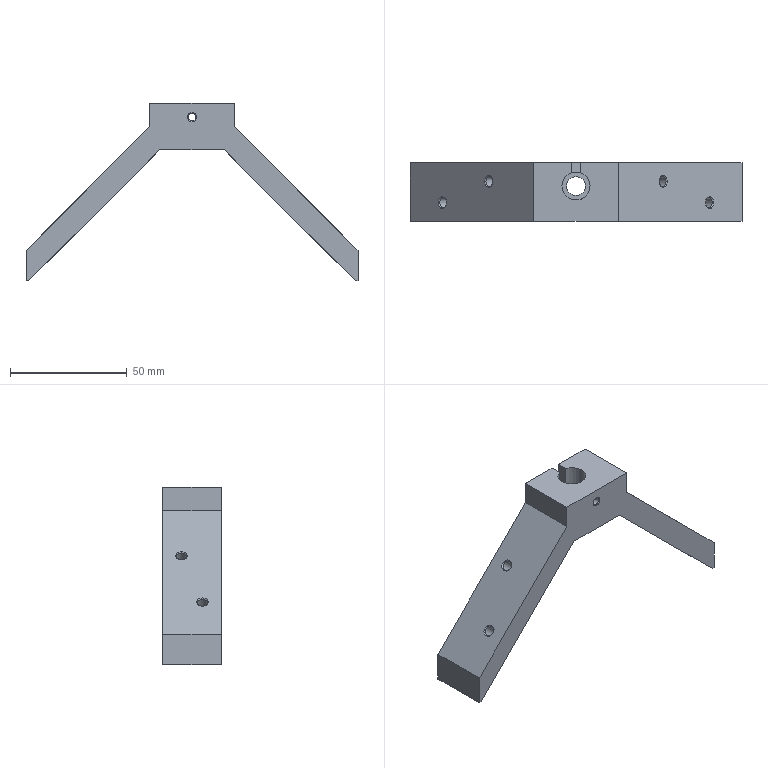Part | NX | features DATUM_CSYS 8, SKETCH 7, SIMPLE HOLE 5, SYMBOLIC_THREAD 5, HOLE PACKAGE 4, EXTRUDE 3, EXTRACT_FACE 2, CBORE_HOLE 1, Instance Feature 1, Mirror Feature 1 | 1 solid | 35 faces | box 142 x 25 x 76 mm | volume 53307 mm3 | plane 18 | cone 9 | cylinder 7 | spline 1 | commonest cylinder face diameters 4.2 x4 3.3 x1 8 x1 12 x1
STEP:
#1=CARTESIAN_POINT('',(2.,12.5,20.));
#2=VERTEX_POINT('',#1);
#3=CARTESIAN_POINT('',(2.,12.5,10.));
#4=VERTEX_POINT('',#3);
#5=CARTESIAN_POINT('',(2.,12.5,20.));
#6=DIRECTION('',(0.,0.,-1.));
#7=VECTOR('',#6,1000.);
#8=LINE('',#5,#7);
#9=EDGE_CURVE('',#2,#4,#8,.T.);
#10=ORIENTED_EDGE('',*,*,#9,.F.);
#11=CARTESIAN_POINT('',(18.,12.5,20.));
#12=VERTEX_POINT('',#11);
#13=CARTESIAN_POINT('',(18.,12.5,20.));
#14=DIRECTION('',(-1.,0.,0.));
#15=VECTOR('',#14,1000.);
#16=LINE('',#13,#15);
#17=EDGE_CURVE('',#12,#2,#16,.T.);
#18=ORIENTED_EDGE('',*,*,#17,.F.);
#19=CARTESIAN_POINT('',(18.,12.5,10.));
#20=VERTEX_POINT('',#19);
#21=CARTESIAN_POINT('',(18.,12.5,20.));
#22=DIRECTION('',(0.,0.,-1.));
#23=VECTOR('',#22,1000.);
#24=LINE('',#21,#23);
#25=EDGE_CURVE('',#12,#20,#24,.T.);
#26=ORIENTED_EDGE('',*,*,#25,.T.);
#27=CARTESIAN_POINT('',(71.,12.5,-43.));
#28=VERTEX_POINT('',#27);
#29=CARTESIAN_POINT('',(71.,12.5,-43.));
#30=DIRECTION('',(-0.7071,0.,0.7071));
#31=VECTOR('',#30,1000.);
#32=LINE('',#29,#31);
#33=EDGE_CURVE('',#28,#20,#32,.T.);
#34=ORIENTED_EDGE('',*,*,#33,.F.);
#35=CARTESIAN_POINT('',(71.,12.5,-56.));
#36=VERTEX_POINT('',#35);
#37=CARTESIAN_POINT('',(71.,12.5,-56.));
#38=DIRECTION('',(0.,0.,1.));
#39=VECTOR('',#38,1000.);
#40=LINE('',#37,#39);
#41=EDGE_CURVE('',#36,#28,#40,.T.);
#42=ORIENTED_EDGE('',*,*,#41,.F.);
#43=CARTESIAN_POINT('',(69.858,12.5,-56.));
#44=VERTEX_POINT('',#43);
#45=CARTESIAN_POINT('',(69.858,12.5,-56.));
#46=DIRECTION('',(1.,0.,0.));
#47=VECTOR('',#46,1000.);
#48=LINE('',#45,#47);
#49=EDGE_CURVE('',#44,#36,#48,.T.);
#50=ORIENTED_EDGE('',*,*,#49,.F.);
#51=CARTESIAN_POINT('',(13.858,12.5,0.));
#52=VERTEX_POINT('',#51);
#53=CARTESIAN_POINT('',(13.858,12.5,0.));
#54=DIRECTION('',(0.7071,0.,-0.7071));
#55=VECTOR('',#54,1000.);
#56=LINE('',#53,#55);
#57=EDGE_CURVE('',#52,#44,#56,.T.);
#58=ORIENTED_EDGE('',*,*,#57,.F.);
#59=CARTESIAN_POINT('',(-13.858,12.5,0.));
#60=VERTEX_POINT('',#59);
#61=CARTESIAN_POINT('',(18.,12.5,0.));
#62=DIRECTION('',(-1.,0.,0.));
#63=VECTOR('',#62,1000.);
#64=LINE('',#61,#63);
#65=EDGE_CURVE('',#52,#60,#64,.T.);
#66=ORIENTED_EDGE('',*,*,#65,.T.);
#67=CARTESIAN_POINT('',(-69.858,12.5,-56.));
#68=VERTEX_POINT('',#67);
#69=CARTESIAN_POINT('',(-69.858,12.5,-56.));
#70=DIRECTION('',(0.7071,0.,0.7071));
#71=VECTOR('',#70,1000.);
#72=LINE('',#69,#71);
#73=EDGE_CURVE('',#68,#60,#72,.T.);
#74=ORIENTED_EDGE('',*,*,#73,.F.);
#75=CARTESIAN_POINT('',(-71.,12.5,-56.));
#76=VERTEX_POINT('',#75);
#77=CARTESIAN_POINT('',(-71.,12.5,-56.));
#78=DIRECTION('',(1.,0.,0.));
#79=VECTOR('',#78,1000.);
#80=LINE('',#77,#79);
#81=EDGE_CURVE('',#76,#68,#80,.T.);
#82=ORIENTED_EDGE('',*,*,#81,.F.);
#83=CARTESIAN_POINT('',(-71.,12.5,-43.));
#84=VERTEX_POINT('',#83);
#85=CARTESIAN_POINT('',(-71.,12.5,-43.));
#86=DIRECTION('',(0.,0.,-1.));
#87=VECTOR('',#86,1000.);
#88=LINE('',#85,#87);
#89=EDGE_CURVE('',#84,#76,#88,.T.);
#90=ORIENTED_EDGE('',*,*,#89,.F.);
#91=CARTESIAN_POINT('',(-18.,12.5,10.));
#92=VERTEX_POINT('',#91);
#93=CARTESIAN_POINT('',(-18.,12.5,10.));
#94=DIRECTION('',(-0.7071,0.,-0.7071));
#95=VECTOR('',#94,1000.);
#96=LINE('',#93,#95);
#97=EDGE_CURVE('',#92,#84,#96,.T.);
#98=ORIENTED_EDGE('',*,*,#97,.F.);
#99=CARTESIAN_POINT('',(-18.,12.5,20.));
#100=VERTEX_POINT('',#99);
#101=CARTESIAN_POINT('',(-18.,12.5,20.));
#102=DIRECTION('',(0.,0.,-1.));
#103=VECTOR('',#102,1000.);
#104=LINE('',#101,#103);
#105=EDGE_CURVE('',#100,#92,#104,.T.);
#106=ORIENTED_EDGE('',*,*,#105,.F.);
#107=CARTESIAN_POINT('',(-2.,12.5,20.));
#108=VERTEX_POINT('',#107);
#109=CARTESIAN_POINT('',(18.,12.5,20.));
#110=DIRECTION('',(-1.,0.,0.));
#111=VECTOR('',#110,1000.);
#112=LINE('',#109,#111);
#113=EDGE_CURVE('',#108,#100,#112,.T.);
#114=ORIENTED_EDGE('',*,*,#113,.F.);
#115=CARTESIAN_POINT('',(-2.,12.5,10.));
#116=VERTEX_POINT('',#115);
#117=CARTESIAN_POINT('',(-2.,12.5,20.));
#118=DIRECTION('',(0.,0.,1.));
#119=VECTOR('',#118,1000.);
#120=LINE('',#117,#119);
#121=EDGE_CURVE('',#116,#108,#120,.T.);
#122=ORIENTED_EDGE('',*,*,#121,.F.);
#123=CARTESIAN_POINT('',(18.,12.5,10.));
#124=DIRECTION('',(1.,0.,0.));
#125=VECTOR('',#124,1000.);
#126=LINE('',#123,#125);
#127=EDGE_CURVE('',#116,#4,#126,.T.);
#128=ORIENTED_EDGE('',*,*,#127,.T.);
#129=EDGE_LOOP('',(#10,#18,#26,#34,#42,#50,#58,#66,#74,#82,#90,#98,#106,#114,#122,#128));
#130=FACE_BOUND('',#129,.T.);
#131=CARTESIAN_POINT('',(18.,12.5,20.));
#132=DIRECTION('',(0.,-1.,0.));
#133=DIRECTION('',(0.,0.,-1.));
#134=AXIS2_PLACEMENT_3D('',#131,#132,#133);
#135=PLANE('',#134);
#136=ADVANCED_FACE('',(#130),#135,.F.);
#137=CARTESIAN_POINT('',(2.,8.157,20.));
#138=VERTEX_POINT('',#137);
#139=CARTESIAN_POINT('',(-2.,8.157,20.));
#140=VERTEX_POINT('',#139);
#141=CARTESIAN_POINT('',(0.,2.5,20.));
#142=DIRECTION('',(0.,0.,-1.));
#143=DIRECTION('',(-1.,0.,0.));
#144=AXIS2_PLACEMENT_3D('',#141,#142,#143);
#145=CIRCLE('',#144,6.);
#146=EDGE_CURVE('',#138,#140,#145,.T.);
#147=ORIENTED_EDGE('',*,*,#146,.T.);
#148=CARTESIAN_POINT('',(-2.,5.4,20.));
#149=DIRECTION('',(0.,1.,0.));
#150=VECTOR('',#149,1000.);
#151=LINE('',#148,#150);
#152=EDGE_CURVE('',#140,#108,#151,.T.);
#153=ORIENTED_EDGE('',*,*,#152,.T.);
#154=ORIENTED_EDGE('',*,*,#113,.T.);
#155=CARTESIAN_POINT('',(-18.,-12.5,20.));
#156=VERTEX_POINT('',#155);
#157=CARTESIAN_POINT('',(-18.,12.5,20.));
#158=DIRECTION('',(0.,-1.,0.));
#159=VECTOR('',#158,1000.);
#160=LINE('',#157,#159);
#161=EDGE_CURVE('',#100,#156,#160,.T.);
#162=ORIENTED_EDGE('',*,*,#161,.T.);
#163=CARTESIAN_POINT('',(18.,-12.5,20.));
#164=VERTEX_POINT('',#163);
#165=CARTESIAN_POINT('',(-18.,-12.5,20.));
#166=DIRECTION('',(1.,0.,0.));
#167=VECTOR('',#166,1000.);
#168=LINE('',#165,#167);
#169=EDGE_CURVE('',#156,#164,#168,.T.);
#170=ORIENTED_EDGE('',*,*,#169,.T.);
#171=CARTESIAN_POINT('',(18.,-12.5,20.));
#172=DIRECTION('',(0.,1.,0.));
#173=VECTOR('',#172,1000.);
#174=LINE('',#171,#173);
#175=EDGE_CURVE('',#164,#12,#174,.T.);
#176=ORIENTED_EDGE('',*,*,#175,.T.);
#177=ORIENTED_EDGE('',*,*,#17,.T.);
#178=CARTESIAN_POINT('',(2.,14.3,20.));
#179=DIRECTION('',(0.,-1.,0.));
#180=VECTOR('',#179,1000.);
#181=LINE('',#178,#180);
#182=EDGE_CURVE('',#2,#138,#181,.T.);
#183=ORIENTED_EDGE('',*,*,#182,.T.);
#184=EDGE_LOOP('',(#147,#153,#154,#162,#170,#176,#177,#183));
#185=FACE_BOUND('',#184,.T.);
#186=CARTESIAN_POINT('',(0.,0.,20.));
#187=DIRECTION('',(0.,0.,1.));
#188=DIRECTION('',(1.,0.,0.));
#189=AXIS2_PLACEMENT_3D('',#186,#187,#188);
#190=PLANE('',#189);
#191=ADVANCED_FACE('',(#185),#190,.T.);
#192=CARTESIAN_POINT('',(-6.,2.5,8.));
#193=VERTEX_POINT('',#192);
#194=CARTESIAN_POINT('',(0.,2.5,8.));
#195=DIRECTION('',(0.,0.,-1.));
#196=DIRECTION('',(-1.,0.,0.));
#197=AXIS2_PLACEMENT_3D('',#194,#195,#196);
#198=CIRCLE('',#197,6.);
#199=EDGE_CURVE('',#193,#193,#198,.F.);
#200=ORIENTED_EDGE('',*,*,#199,.F.);
#201=EDGE_LOOP('',(#200));
#202=FACE_BOUND('',#201,.T.);
#203=CARTESIAN_POINT('',(0.,-3.5,16.061));
#204=VERTEX_POINT('',#203);
#205=CARTESIAN_POINT('',(1.275,-3.383,15.709));
#206=CARTESIAN_POINT('',(0.03766,-3.572,16.278));
#207=CARTESIAN_POINT('',(-1.209,-3.398,15.751));
#208=CARTESIAN_POINT('',(-1.79,-3.229,14.866));
#209=CARTESIAN_POINT('',(-1.965,-3.169,14.045));
#210=CARTESIAN_POINT('',(-1.824,-3.218,13.231));
#211=CARTESIAN_POINT('',(-1.288,-3.378,12.314));
#212=CARTESIAN_POINT('',(-0.07795,-3.571,11.724));
#213=CARTESIAN_POINT('',(1.193,-3.403,12.223));
#214=CARTESIAN_POINT('',(1.789,-3.229,13.134));
#215=CARTESIAN_POINT('',(1.965,-3.169,13.957));
#216=CARTESIAN_POINT('',(1.824,-3.218,14.771));
#217=CARTESIAN_POINT('',(1.275,-3.383,15.709));
#218=CARTESIAN_POINT('',(0.03766,-3.572,16.278));
#219=CARTESIAN_POINT('',(-1.209,-3.398,15.751));
#220=B_SPLINE_CURVE_WITH_KNOTS('',3,(#205,#206,#207,#208,#209,#210,#211,#212,#213,#214,#215,#216,#217,#218,#219),.UNSPECIFIED.,.T.,.F.,(1,1,1,1,1,1,1,1,1,1,1,1,1,1,1,1,1,1,1),(-0.2533,-0.1908,-0.1283,0.,0.1187,0.1841,0.2467,0.3092,0.3717,0.4936,0.6184,0.684,0.7467,0.8092,0.8717,1.,1.119,1.184,1.247),.UNSPECIFIED.);
#221=EDGE_CURVE('',#204,#204,#220,.T.);
#222=ORIENTED_EDGE('',*,*,#221,.T.);
#223=EDGE_LOOP('',(#222));
#224=FACE_BOUND('',#223,.T.);
#225=CARTESIAN_POINT('',(2.,8.157,10.));
#226=VERTEX_POINT('',#225);
#227=CARTESIAN_POINT('',(2.,8.157,20.));
#228=DIRECTION('',(0.,0.,-1.));
#229=VECTOR('',#228,1000.);
#230=LINE('',#227,#229);
#231=EDGE_CURVE('',#226,#138,#230,.F.);
#232=ORIENTED_EDGE('',*,*,#231,.F.);
#233=CARTESIAN_POINT('',(-2.,8.157,10.));
#234=VERTEX_POINT('',#233);
#235=CARTESIAN_POINT('',(0.,2.5,10.));
#236=DIRECTION('',(0.,0.,-1.));
#237=DIRECTION('',(-1.,0.,0.));
#238=AXIS2_PLACEMENT_3D('',#235,#236,#237);
#239=CIRCLE('',#238,6.);
#240=EDGE_CURVE('',#226,#234,#239,.F.);
#241=ORIENTED_EDGE('',*,*,#240,.T.);
#242=CARTESIAN_POINT('',(-2.,8.157,20.));
#243=DIRECTION('',(0.,0.,-1.));
#244=VECTOR('',#243,1000.);
#245=LINE('',#242,#244);
#246=EDGE_CURVE('',#140,#234,#245,.T.);
#247=ORIENTED_EDGE('',*,*,#246,.F.);
#248=ORIENTED_EDGE('',*,*,#146,.F.);
#249=EDGE_LOOP('',(#232,#241,#247,#248));
#250=FACE_BOUND('',#249,.T.);
#251=CARTESIAN_POINT('',(0.,2.5,20.));
#252=DIRECTION('',(0.,0.,-1.));
#253=DIRECTION('',(-1.,0.,0.));
#254=AXIS2_PLACEMENT_3D('',#251,#252,#253);
#255=CYLINDRICAL_SURFACE('',#254,6.);
#256=ADVANCED_FACE('',(#202,#224,#250),#255,.F.);
#257=CARTESIAN_POINT('',(4.,2.5,0.));
#258=VERTEX_POINT('',#257);
#259=CARTESIAN_POINT('',(0.,2.5,0.));
#260=DIRECTION('',(0.,0.,1.));
#261=DIRECTION('',(1.,0.,0.));
#262=AXIS2_PLACEMENT_3D('',#259,#260,#261);
#263=CIRCLE('',#262,4.);
#264=EDGE_CURVE('',#258,#258,#263,.T.);
#265=ORIENTED_EDGE('',*,*,#264,.T.);
#266=EDGE_LOOP('',(#265));
#267=FACE_BOUND('',#266,.T.);
#268=CARTESIAN_POINT('',(13.858,-12.5,0.));
#269=VERTEX_POINT('',#268);
#270=CARTESIAN_POINT('',(13.858,-12.5,0.));
#271=DIRECTION('',(0.,1.,0.));
#272=VECTOR('',#271,1000.);
#273=LINE('',#270,#272);
#274=EDGE_CURVE('',#269,#52,#273,.T.);
#275=ORIENTED_EDGE('',*,*,#274,.F.);
#276=CARTESIAN_POINT('',(-13.858,-12.5,0.));
#277=VERTEX_POINT('',#276);
#278=CARTESIAN_POINT('',(-18.,-12.5,0.));
#279=DIRECTION('',(1.,0.,0.));
#280=VECTOR('',#279,1000.);
#281=LINE('',#278,#280);
#282=EDGE_CURVE('',#277,#269,#281,.T.);
#283=ORIENTED_EDGE('',*,*,#282,.F.);
#284=CARTESIAN_POINT('',(-13.858,-12.5,0.));
#285=DIRECTION('',(0.,1.,0.));
#286=VECTOR('',#285,1000.);
#287=LINE('',#284,#286);
#288=EDGE_CURVE('',#277,#60,#287,.T.);
#289=ORIENTED_EDGE('',*,*,#288,.T.);
#290=ORIENTED_EDGE('',*,*,#65,.F.);
#291=EDGE_LOOP('',(#275,#283,#289,#290));
#292=FACE_BOUND('',#291,.T.);
#293=CARTESIAN_POINT('',(0.,0.,0.));
#294=DIRECTION('',(0.,0.,1.));
#295=DIRECTION('',(1.,0.,0.));
#296=AXIS2_PLACEMENT_3D('',#293,#294,#295);
#297=PLANE('',#296);
#298=ADVANCED_FACE('',(#267,#292),#297,.F.);
#299=CARTESIAN_POINT('',(18.,-12.5,10.));
#300=VERTEX_POINT('',#299);
#301=CARTESIAN_POINT('',(18.,-12.5,10.));
#302=DIRECTION('',(0.,1.,0.));
#303=VECTOR('',#302,1000.);
#304=LINE('',#301,#303);
#305=EDGE_CURVE('',#300,#20,#304,.T.);
#306=ORIENTED_EDGE('',*,*,#305,.T.);
#307=ORIENTED_EDGE('',*,*,#25,.F.);
#308=ORIENTED_EDGE('',*,*,#175,.F.);
#309=CARTESIAN_POINT('',(18.,-12.5,20.));
#310=DIRECTION('',(0.,0.,-1.));
#311=VECTOR('',#310,1000.);
#312=LINE('',#309,#311);
#313=EDGE_CURVE('',#164,#300,#312,.T.);
#314=ORIENTED_EDGE('',*,*,#313,.T.);
#315=EDGE_LOOP('',(#306,#307,#308,#314));
#316=FACE_BOUND('',#315,.T.);
#317=CARTESIAN_POINT('',(18.,-12.5,20.));
#318=DIRECTION('',(-1.,0.,0.));
#319=DIRECTION('',(0.,0.,1.));
#320=AXIS2_PLACEMENT_3D('',#317,#318,#319);
#321=PLANE('',#320);
#322=ADVANCED_FACE('',(#316),#321,.F.);
#323=CARTESIAN_POINT('',(-18.,-12.5,10.));
#324=VERTEX_POINT('',#323);
#325=CARTESIAN_POINT('',(-18.,-12.5,10.));
#326=DIRECTION('',(0.,1.,0.));
#327=VECTOR('',#326,1000.);
#328=LINE('',#325,#327);
#329=EDGE_CURVE('',#324,#92,#328,.T.);
#330=ORIENTED_EDGE('',*,*,#329,.F.);
#331=CARTESIAN_POINT('',(-18.,-12.5,20.));
#332=DIRECTION('',(0.,0.,-1.));
#333=VECTOR('',#332,1000.);
#334=LINE('',#331,#333);
#335=EDGE_CURVE('',#156,#324,#334,.T.);
#336=ORIENTED_EDGE('',*,*,#335,.F.);
#337=ORIENTED_EDGE('',*,*,#161,.F.);
#338=ORIENTED_EDGE('',*,*,#105,.T.);
#339=EDGE_LOOP('',(#330,#336,#337,#338));
#340=FACE_BOUND('',#339,.T.);
#341=CARTESIAN_POINT('',(-18.,12.5,20.));
#342=DIRECTION('',(1.,0.,0.));
#343=DIRECTION('',(0.,0.,-1.));
#344=AXIS2_PLACEMENT_3D('',#341,#342,#343);
#345=PLANE('',#344);
#346=ADVANCED_FACE('',(#340),#345,.F.);
#347=CARTESIAN_POINT('',(0.,-12.5,16.));
#348=VERTEX_POINT('',#347);
#349=CARTESIAN_POINT('',(0.,-12.5,14.));
#350=DIRECTION('',(0.,1.,0.));
#351=DIRECTION('',(0.,0.,1.));
#352=AXIS2_PLACEMENT_3D('',#349,#350,#351);
#353=CIRCLE('',#352,2.);
#354=EDGE_CURVE('',#348,#348,#353,.T.);
#355=ORIENTED_EDGE('',*,*,#354,.T.);
#356=EDGE_LOOP('',(#355));
#357=FACE_BOUND('',#356,.T.);
#358=ORIENTED_EDGE('',*,*,#282,.T.);
#359=CARTESIAN_POINT('',(69.858,-12.5,-56.));
#360=VERTEX_POINT('',#359);
#361=CARTESIAN_POINT('',(13.858,-12.5,0.));
#362=DIRECTION('',(0.7071,0.,-0.7071));
#363=VECTOR('',#362,1000.);
#364=LINE('',#361,#363);
#365=EDGE_CURVE('',#269,#360,#364,.T.);
#366=ORIENTED_EDGE('',*,*,#365,.T.);
#367=CARTESIAN_POINT('',(71.,-12.5,-56.));
#368=VERTEX_POINT('',#367);
#369=CARTESIAN_POINT('',(69.858,-12.5,-56.));
#370=DIRECTION('',(1.,0.,0.));
#371=VECTOR('',#370,1000.);
#372=LINE('',#369,#371);
#373=EDGE_CURVE('',#360,#368,#372,.T.);
#374=ORIENTED_EDGE('',*,*,#373,.T.);
#375=CARTESIAN_POINT('',(71.,-12.5,-43.));
#376=VERTEX_POINT('',#375);
#377=CARTESIAN_POINT('',(71.,-12.5,-56.));
#378=DIRECTION('',(0.,0.,1.));
#379=VECTOR('',#378,1000.);
#380=LINE('',#377,#379);
#381=EDGE_CURVE('',#368,#376,#380,.T.);
#382=ORIENTED_EDGE('',*,*,#381,.T.);
#383=CARTESIAN_POINT('',(71.,-12.5,-43.));
#384=DIRECTION('',(-0.7071,0.,0.7071));
#385=VECTOR('',#384,1000.);
#386=LINE('',#383,#385);
#387=EDGE_CURVE('',#376,#300,#386,.T.);
#388=ORIENTED_EDGE('',*,*,#387,.T.);
#389=ORIENTED_EDGE('',*,*,#313,.F.);
#390=ORIENTED_EDGE('',*,*,#169,.F.);
#391=ORIENTED_EDGE('',*,*,#335,.T.);
#392=CARTESIAN_POINT('',(-71.,-12.5,-43.));
#393=VERTEX_POINT('',#392);
#394=CARTESIAN_POINT('',(-18.,-12.5,10.));
#395=DIRECTION('',(-0.7071,0.,-0.7071));
#396=VECTOR('',#395,1000.);
#397=LINE('',#394,#396);
#398=EDGE_CURVE('',#324,#393,#397,.T.);
#399=ORIENTED_EDGE('',*,*,#398,.T.);
#400=CARTESIAN_POINT('',(-71.,-12.5,-56.));
#401=VERTEX_POINT('',#400);
#402=CARTESIAN_POINT('',(-71.,-12.5,-43.));
#403=DIRECTION('',(0.,0.,-1.));
#404=VECTOR('',#403,1000.);
#405=LINE('',#402,#404);
#406=EDGE_CURVE('',#393,#401,#405,.T.);
#407=ORIENTED_EDGE('',*,*,#406,.T.);
#408=CARTESIAN_POINT('',(-69.858,-12.5,-56.));
#409=VERTEX_POINT('',#408);
#410=CARTESIAN_POINT('',(-71.,-12.5,-56.));
#411=DIRECTION('',(1.,0.,0.));
#412=VECTOR('',#411,1000.);
#413=LINE('',#410,#412);
#414=EDGE_CURVE('',#401,#409,#413,.T.);
#415=ORIENTED_EDGE('',*,*,#414,.T.);
#416=CARTESIAN_POINT('',(-69.858,-12.5,-56.));
#417=DIRECTION('',(0.7071,0.,0.7071));
#418=VECTOR('',#417,1000.);
#419=LINE('',#416,#418);
#420=EDGE_CURVE('',#409,#277,#419,.T.);
#421=ORIENTED_EDGE('',*,*,#420,.T.);
#422=EDGE_LOOP('',(#358,#366,#374,#382,#388,#389,#390,#391,#399,#407,#415,#421));
#423=FACE_BOUND('',#422,.T.);
#424=CARTESIAN_POINT('',(-18.,-12.5,20.));
#425=DIRECTION('',(0.,1.,0.));
#426=DIRECTION('',(0.,0.,1.));
#427=AXIS2_PLACEMENT_3D('',#424,#425,#426);
#428=PLANE('',#427);
#429=ADVANCED_FACE('',(#357,#423),#428,.F.);
#430=ORIENTED_EDGE('',*,*,#89,.T.);
#431=CARTESIAN_POINT('',(-71.,-12.5,-56.));
#432=DIRECTION('',(0.,1.,0.));
#433=VECTOR('',#432,1000.);
#434=LINE('',#431,#433);
#435=EDGE_CURVE('',#401,#76,#434,.T.);
#436=ORIENTED_EDGE('',*,*,#435,.F.);
#437=ORIENTED_EDGE('',*,*,#406,.F.);
#438=CARTESIAN_POINT('',(-71.,-12.5,-43.));
#439=DIRECTION('',(0.,1.,0.));
#440=VECTOR('',#439,1000.);
#441=LINE('',#438,#440);
#442=EDGE_CURVE('',#393,#84,#441,.T.);
#443=ORIENTED_EDGE('',*,*,#442,.T.);
#444=EDGE_LOOP('',(#430,#436,#437,#443));
#445=FACE_BOUND('',#444,.T.);
#446=CARTESIAN_POINT('',(-71.,-12.5,-43.));
#447=DIRECTION('',(1.,0.,0.));
#448=DIRECTION('',(0.,0.,-1.));
#449=AXIS2_PLACEMENT_3D('',#446,#447,#448);
#450=PLANE('',#449);
#451=ADVANCED_FACE('',(#445),#450,.F.);
#452=ORIENTED_EDGE('',*,*,#81,.T.);
#453=CARTESIAN_POINT('',(-69.858,-12.5,-56.));
#454=DIRECTION('',(0.,1.,0.));
#455=VECTOR('',#454,1000.);
#456=LINE('',#453,#455);
#457=EDGE_CURVE('',#409,#68,#456,.T.);
#458=ORIENTED_EDGE('',*,*,#457,.F.);
#459=ORIENTED_EDGE('',*,*,#414,.F.);
#460=ORIENTED_EDGE('',*,*,#435,.T.);
#461=EDGE_LOOP('',(#452,#458,#459,#460));
#462=FACE_BOUND('',#461,.T.);
#463=CARTESIAN_POINT('',(-71.,-12.5,-56.));
#464=DIRECTION('',(0.,0.,1.));
#465=DIRECTION('',(1.,0.,0.));
#466=AXIS2_PLACEMENT_3D('',#463,#464,#465);
#467=PLANE('',#466);
#468=ADVANCED_FACE('',(#462),#467,.F.);
#469=CARTESIAN_POINT('',(-48.291,-4.5,-34.433));
#470=VERTEX_POINT('',#469);
#471=CARTESIAN_POINT('',(-50.059,-4.5,-36.201));
#472=DIRECTION('',(-0.7071,0.,0.7071));
#473=DIRECTION('',(0.7071,0.,0.7071));
#474=AXIS2_PLACEMENT_3D('',#471,#472,#473);
#475=CIRCLE('',#474,2.5);
#476=EDGE_CURVE('',#470,#470,#475,.T.);
#477=ORIENTED_EDGE('',*,*,#476,.T.);
#478=EDGE_LOOP('',(#477));
#479=FACE_BOUND('',#478,.T.);
#480=CARTESIAN_POINT('',(-28.492,4.5,-14.634));
#481=VERTEX_POINT('',#480);
#482=CARTESIAN_POINT('',(-30.26,4.5,-16.402));
#483=DIRECTION('',(-0.7071,0.,0.7071));
#484=DIRECTION('',(0.7071,0.,0.7071));
#485=AXIS2_PLACEMENT_3D('',#482,#483,#484);
#486=CIRCLE('',#485,2.5);
#487=EDGE_CURVE('',#481,#481,#486,.T.);
#488=ORIENTED_EDGE('',*,*,#487,.T.);
#489=EDGE_LOOP('',(#488));
#490=FACE_BOUND('',#489,.T.);
#491=ORIENTED_EDGE('',*,*,#73,.T.);
#492=ORIENTED_EDGE('',*,*,#288,.F.);
#493=ORIENTED_EDGE('',*,*,#420,.F.);
#494=ORIENTED_EDGE('',*,*,#457,.T.);
#495=EDGE_LOOP('',(#491,#492,#493,#494));
#496=FACE_BOUND('',#495,.T.);
#497=CARTESIAN_POINT('',(-69.858,-12.5,-56.));
#498=DIRECTION('',(-0.7071,0.,0.7071));
#499=DIRECTION('',(0.7071,0.,0.7071));
#500=AXIS2_PLACEMENT_3D('',#497,#498,#499);
#501=PLANE('',#500);
#502=ADVANCED_FACE('',(#479,#490,#496),#501,.F.);
#503=CARTESIAN_POINT('',(-58.898,-4.5,-30.898));
#504=VERTEX_POINT('',#503);
#505=CARTESIAN_POINT('',(-57.13,-4.5,-29.13));
#506=DIRECTION('',(0.7071,0.,-0.7071));
#507=DIRECTION('',(-0.7071,0.,-0.7071));
#508=AXIS2_PLACEMENT_3D('',#505,#506,#507);
#509=CIRCLE('',#508,2.5);
#510=EDGE_CURVE('',#504,#504,#509,.T.);
#511=ORIENTED_EDGE('',*,*,#510,.T.);
#512=EDGE_LOOP('',(#511));
#513=FACE_BOUND('',#512,.T.);
#514=CARTESIAN_POINT('',(-39.099,4.5,-11.099));
#515=VERTEX_POINT('',#514);
#516=CARTESIAN_POINT('',(-37.331,4.5,-9.331));
#517=DIRECTION('',(0.7071,0.,-0.7071));
#518=DIRECTION('',(-0.7071,0.,-0.7071));
#519=AXIS2_PLACEMENT_3D('',#516,#517,#518);
#520=CIRCLE('',#519,2.5);
#521=EDGE_CURVE('',#515,#515,#520,.T.);
#522=ORIENTED_EDGE('',*,*,#521,.T.);
#523=EDGE_LOOP('',(#522));
#524=FACE_BOUND('',#523,.T.);
#525=ORIENTED_EDGE('',*,*,#97,.T.);
#526=ORIENTED_EDGE('',*,*,#442,.F.);
#527=ORIENTED_EDGE('',*,*,#398,.F.);
#528=ORIENTED_EDGE('',*,*,#329,.T.);
#529=EDGE_LOOP('',(#525,#526,#527,#528));
#530=FACE_BOUND('',#529,.T.);
#531=CARTESIAN_POINT('',(-18.,-12.5,10.));
#532=DIRECTION('',(0.7071,0.,-0.7071));
#533=DIRECTION('',(-0.7071,0.,-0.7071));
#534=AXIS2_PLACEMENT_3D('',#531,#532,#533);
#535=PLANE('',#534);
#536=ADVANCED_FACE('',(#513,#524,#530),#535,.F.);
#537=CARTESIAN_POINT('',(51.827,-4.5,-37.969));
#538=VERTEX_POINT('',#537);
#539=CARTESIAN_POINT('',(50.059,-4.5,-36.201));
#540=DIRECTION('',(0.7071,0.,0.7071));
#541=DIRECTION('',(0.7071,0.,-0.7071));
#542=AXIS2_PLACEMENT_3D('',#539,#540,#541);
#543=CIRCLE('',#542,2.5);
#544=EDGE_CURVE('',#538,#538,#543,.T.);
#545=ORIENTED_EDGE('',*,*,#544,.T.);
#546=EDGE_LOOP('',(#545));
#547=FACE_BOUND('',#546,.T.);
#548=CARTESIAN_POINT('',(32.028,4.5,-18.17));
#549=VERTEX_POINT('',#548);
#550=CARTESIAN_POINT('',(30.26,4.5,-16.402));
#551=DIRECTION('',(0.7071,0.,0.7071));
#552=DIRECTION('',(0.7071,0.,-0.7071));
#553=AXIS2_PLACEMENT_3D('',#550,#551,#552);
#554=CIRCLE('',#553,2.5);
#555=EDGE_CURVE('',#549,#549,#554,.T.);
#556=ORIENTED_EDGE('',*,*,#555,.T.);
#557=EDGE_LOOP('',(#556));
#558=FACE_BOUND('',#557,.T.);
#559=ORIENTED_EDGE('',*,*,#57,.T.);
#560=CARTESIAN_POINT('',(69.858,-12.5,-56.));
#561=DIRECTION('',(0.,1.,0.));
#562=VECTOR('',#561,1000.);
#563=LINE('',#560,#562);
#564=EDGE_CURVE('',#360,#44,#563,.T.);
#565=ORIENTED_EDGE('',*,*,#564,.F.);
#566=ORIENTED_EDGE('',*,*,#365,.F.);
#567=ORIENTED_EDGE('',*,*,#274,.T.);
#568=EDGE_LOOP('',(#559,#565,#566,#567));
#569=FACE_BOUND('',#568,.T.);
#570=CARTESIAN_POINT('',(13.858,-12.5,0.));
#571=DIRECTION('',(0.7071,0.,0.7071));
#572=DIRECTION('',(0.7071,0.,-0.7071));
#573=AXIS2_PLACEMENT_3D('',#570,#571,#572);
#574=PLANE('',#573);
#575=ADVANCED_FACE('',(#547,#558,#569),#574,.F.);
#576=ORIENTED_EDGE('',*,*,#49,.T.);
#577=CARTESIAN_POINT('',(71.,-12.5,-56.));
#578=DIRECTION('',(0.,1.,0.));
#579=VECTOR('',#578,1000.);
#580=LINE('',#577,#579);
#581=EDGE_CURVE('',#368,#36,#580,.T.);
#582=ORIENTED_EDGE('',*,*,#581,.F.);
#583=ORIENTED_EDGE('',*,*,#373,.F.);
#584=ORIENTED_EDGE('',*,*,#564,.T.);
#585=EDGE_LOOP('',(#576,#582,#583,#584));
#586=FACE_BOUND('',#585,.T.);
#587=CARTESIAN_POINT('',(69.858,-12.5,-56.));
#588=DIRECTION('',(0.,0.,1.));
#589=DIRECTION('',(1.,0.,0.));
#590=AXIS2_PLACEMENT_3D('',#587,#588,#589);
#591=PLANE('',#590);
#592=ADVANCED_FACE('',(#586),#591,.F.);
#593=ORIENTED_EDGE('',*,*,#41,.T.);
#594=CARTESIAN_POINT('',(71.,-12.5,-43.));
#595=DIRECTION('',(0.,1.,0.));
#596=VECTOR('',#595,1000.);
#597=LINE('',#594,#596);
#598=EDGE_CURVE('',#376,#28,#597,.T.);
#599=ORIENTED_EDGE('',*,*,#598,.F.);
#600=ORIENTED_EDGE('',*,*,#381,.F.);
#601=ORIENTED_EDGE('',*,*,#581,.T.);
#602=EDGE_LOOP('',(#593,#599,#600,#601));
#603=FACE_BOUND('',#602,.T.);
#604=CARTESIAN_POINT('',(71.,-12.5,-56.));
#605=DIRECTION('',(-1.,0.,0.));
#606=DIRECTION('',(0.,0.,1.));
#607=AXIS2_PLACEMENT_3D('',#604,#605,#606);
#608=PLANE('',#607);
#609=ADVANCED_FACE('',(#603),#608,.F.);
#610=CARTESIAN_POINT('',(55.362,-4.5,-27.362));
#611=VERTEX_POINT('',#610);
#612=CARTESIAN_POINT('',(57.13,-4.5,-29.13));
#613=DIRECTION('',(-0.7071,0.,-0.7071));
#614=DIRECTION('',(-0.7071,0.,0.7071));
#615=AXIS2_PLACEMENT_3D('',#612,#613,#614);
#616=CIRCLE('',#615,2.5);
#617=EDGE_CURVE('',#611,#611,#616,.T.);
#618=ORIENTED_EDGE('',*,*,#617,.T.);
#619=EDGE_LOOP('',(#618));
#620=FACE_BOUND('',#619,.T.);
#621=CARTESIAN_POINT('',(35.563,4.5,-7.563));
#622=VERTEX_POINT('',#621);
#623=CARTESIAN_POINT('',(37.331,4.5,-9.331));
#624=DIRECTION('',(-0.7071,0.,-0.7071));
#625=DIRECTION('',(-0.7071,0.,0.7071));
#626=AXIS2_PLACEMENT_3D('',#623,#624,#625);
#627=CIRCLE('',#626,2.5);
#628=EDGE_CURVE('',#622,#622,#627,.T.);
#629=ORIENTED_EDGE('',*,*,#628,.T.);
#630=EDGE_LOOP('',(#629));
#631=FACE_BOUND('',#630,.T.);
#632=ORIENTED_EDGE('',*,*,#33,.T.);
#633=ORIENTED_EDGE('',*,*,#305,.F.);
#634=ORIENTED_EDGE('',*,*,#387,.F.);
#635=ORIENTED_EDGE('',*,*,#598,.T.);
#636=EDGE_LOOP('',(#632,#633,#634,#635));
#637=FACE_BOUND('',#636,.T.);
#638=CARTESIAN_POINT('',(71.,-12.5,-43.));
#639=DIRECTION('',(-0.7071,0.,-0.7071));
#640=DIRECTION('',(-0.7071,0.,0.7071));
#641=AXIS2_PLACEMENT_3D('',#638,#639,#640);
#642=PLANE('',#641);
#643=ADVANCED_FACE('',(#620,#631,#637),#642,.F.);
#644=CARTESIAN_POINT('',(-4.,2.5,8.));
#645=VERTEX_POINT('',#644);
#646=CARTESIAN_POINT('',(0.,2.5,8.));
#647=DIRECTION('',(0.,0.,-1.));
#648=DIRECTION('',(-1.,0.,0.));
#649=AXIS2_PLACEMENT_3D('',#646,#647,#648);
#650=CIRCLE('',#649,4.);
#651=EDGE_CURVE('',#645,#645,#650,.F.);
#652=ORIENTED_EDGE('',*,*,#651,.T.);
#653=EDGE_LOOP('',(#652));
#654=FACE_BOUND('',#653,.T.);
#655=ORIENTED_EDGE('',*,*,#264,.F.);
#656=EDGE_LOOP('',(#655));
#657=FACE_BOUND('',#656,.T.);
#658=CARTESIAN_POINT('',(0.,2.5,-107.608));
#659=DIRECTION('',(0.,0.,-1.));
#660=DIRECTION('',(-1.,0.,0.));
#661=AXIS2_PLACEMENT_3D('',#658,#659,#660);
#662=CYLINDRICAL_SURFACE('',#661,4.);
#663=ADVANCED_FACE('',(#654,#657),#662,.F.);
#664=ORIENTED_EDGE('',*,*,#651,.F.);
#665=EDGE_LOOP('',(#664));
#666=FACE_BOUND('',#665,.T.);
#667=ORIENTED_EDGE('',*,*,#199,.T.);
#668=EDGE_LOOP('',(#667));
#669=FACE_BOUND('',#668,.T.);
#670=CARTESIAN_POINT('',(0.,2.5,8.));
#671=DIRECTION('',(0.,0.,-1.));
#672=DIRECTION('',(-1.,0.,0.));
#673=AXIS2_PLACEMENT_3D('',#670,#671,#672);
#674=PLANE('',#673);
#675=ADVANCED_FACE('',(#666,#669),#674,.F.);
#676=CARTESIAN_POINT('',(0.,-3.964,15.65));
#677=VERTEX_POINT('',#676);
#678=CARTESIAN_POINT('',(-0.5682,-3.938,15.603));
#679=CARTESIAN_POINT('',(-0.01754,-3.976,15.672));
#680=CARTESIAN_POINT('',(0.5095,-3.941,15.608));
#681=CARTESIAN_POINT('',(1.153,-3.816,15.269));
#682=CARTESIAN_POINT('',(1.594,-3.659,14.59));
#683=CARTESIAN_POINT('',(1.668,-3.615,14.042));
#684=CARTESIAN_POINT('',(1.628,-3.643,13.547));
#685=CARTESIAN_POINT('',(1.28,-3.776,12.853));
#686=CARTESIAN_POINT('',(0.6063,-3.931,12.414));
#687=CARTESIAN_POINT('',(0.04585,-3.975,12.328));
#688=CARTESIAN_POINT('',(-0.4702,-3.947,12.378));
#689=CARTESIAN_POINT('',(-1.143,-3.82,12.716));
#690=CARTESIAN_POINT('',(-1.594,-3.659,13.408));
#691=CARTESIAN_POINT('',(-1.668,-3.615,13.959));
#692=CARTESIAN_POINT('',(-1.628,-3.643,14.453));
#693=CARTESIAN_POINT('',(-1.275,-3.778,15.159));
#694=CARTESIAN_POINT('',(-0.5682,-3.938,15.603));
#695=CARTESIAN_POINT('',(-0.01754,-3.976,15.672));
#696=CARTESIAN_POINT('',(0.5095,-3.941,15.608));
#697=B_SPLINE_CURVE_WITH_KNOTS('',3,(#678,#679,#680,#681,#682,#683,#684,#685,#686,#687,#688,#689,#690,#691,#692,#693,#694,#695,#696),.UNSPECIFIED.,.T.,.F.,(1,1,1,1,1,1,1,1,1,1,1,1,1,1,1,1,1,1,1,1,1,1,1),(-0.1941,-0.1316,-0.06579,0.,0.05937,0.1187,0.1811,0.2434,0.3059,0.3684,0.4309,0.4934,0.5559,0.6184,0.6809,0.7434,0.8059,0.8684,0.9342,1.,1.059,1.119,1.181),.UNSPECIFIED.);
#698=EDGE_CURVE('',#677,#677,#697,.T.);
#699=ORIENTED_EDGE('',*,*,#698,.T.);
#700=EDGE_LOOP('',(#699));
#701=FACE_BOUND('',#700,.T.);
#702=CARTESIAN_POINT('',(0.,-12.15,15.65));
#703=VERTEX_POINT('',#702);
#704=CARTESIAN_POINT('',(0.,-12.15,14.));
#705=DIRECTION('',(0.,1.,0.));
#706=DIRECTION('',(0.,0.,1.));
#707=AXIS2_PLACEMENT_3D('',#704,#705,#706);
#708=CIRCLE('',#707,1.65);
#709=EDGE_CURVE('',#703,#703,#708,.F.);
#710=ORIENTED_EDGE('',*,*,#709,.T.);
#711=EDGE_LOOP('',(#710));
#712=FACE_BOUND('',#711,.T.);
#713=CARTESIAN_POINT('',(0.,-12.5,14.));
#714=DIRECTION('',(0.,1.,0.));
#715=DIRECTION('',(0.,0.,1.));
#716=AXIS2_PLACEMENT_3D('',#713,#714,#715);
#717=CYLINDRICAL_SURFACE('',#716,1.65);
#718=ADVANCED_FACE('',(#701,#712),#717,.F.);
#719=ORIENTED_EDGE('',*,*,#709,.F.);
#720=EDGE_LOOP('',(#719));
#721=FACE_BOUND('',#720,.T.);
#722=ORIENTED_EDGE('',*,*,#354,.F.);
#723=EDGE_LOOP('',(#722));
#724=FACE_BOUND('',#723,.T.);
#725=CARTESIAN_POINT('',(0.,-12.5,14.));
#726=DIRECTION('',(0.,-1.,0.));
#727=DIRECTION('',(0.,0.,-1.));
#728=AXIS2_PLACEMENT_3D('',#725,#726,#727);
#729=CONICAL_SURFACE('',#728,2.,0.7854);
#730=ADVANCED_FACE('',(#721,#724),#729,.F.);
#731=ORIENTED_EDGE('',*,*,#698,.F.);
#732=EDGE_LOOP('',(#731));
#733=FACE_BOUND('',#732,.T.);
#734=ORIENTED_EDGE('',*,*,#221,.F.);
#735=EDGE_LOOP('',(#734));
#736=FACE_BOUND('',#735,.T.);
#737=CARTESIAN_POINT('',(0.5058,-3.5,16.061));
#738=CARTESIAN_POINT('',(-0.5058,-3.5,16.061));
#739=CARTESIAN_POINT('',(-1.002,-3.428,15.835));
#740=CARTESIAN_POINT('',(-1.705,-3.263,15.078));
#741=CARTESIAN_POINT('',(-1.913,-3.187,14.545));
#742=CARTESIAN_POINT('',(-1.913,-3.187,13.456));
#743=CARTESIAN_POINT('',(-1.704,-3.263,12.921));
#744=CARTESIAN_POINT('',(-1.,-3.429,12.163));
#745=CARTESIAN_POINT('',(-0.5054,-3.5,11.939));
#746=CARTESIAN_POINT('',(0.5059,-3.5,11.939));
#747=CARTESIAN_POINT('',(1.002,-3.428,12.164));
#748=CARTESIAN_POINT('',(1.705,-3.263,12.923));
#749=CARTESIAN_POINT('',(1.913,-3.187,13.456));
#750=CARTESIAN_POINT('',(1.913,-3.187,14.546));
#751=CARTESIAN_POINT('',(1.704,-3.263,15.079));
#752=CARTESIAN_POINT('',(1.001,-3.428,15.836));
#753=CARTESIAN_POINT('',(0.5058,-3.5,16.061));
#754=CARTESIAN_POINT('',(-0.5058,-3.5,16.061));
#755=CARTESIAN_POINT('',(0.4363,-3.964,15.65));
#756=CARTESIAN_POINT('',(-0.4363,-3.964,15.65));
#757=CARTESIAN_POINT('',(-0.8643,-3.886,15.469));
#758=CARTESIAN_POINT('',(-1.471,-3.708,14.863));
#759=CARTESIAN_POINT('',(-1.65,-3.626,14.437));
#760=CARTESIAN_POINT('',(-1.65,-3.626,13.564));
#761=CARTESIAN_POINT('',(-1.47,-3.708,13.136));
#762=CARTESIAN_POINT('',(-0.8629,-3.887,12.529));
#763=CARTESIAN_POINT('',(-0.4359,-3.964,12.35));
#764=CARTESIAN_POINT('',(0.4364,-3.964,12.35));
#765=CARTESIAN_POINT('',(0.8639,-3.886,12.53));
#766=CARTESIAN_POINT('',(1.47,-3.708,13.138));
#767=CARTESIAN_POINT('',(1.65,-3.626,13.564));
#768=CARTESIAN_POINT('',(1.65,-3.626,14.437));
#769=CARTESIAN_POINT('',(1.47,-3.708,14.864));
#770=CARTESIAN_POINT('',(0.8631,-3.886,15.47));
#771=CARTESIAN_POINT('',(0.4363,-3.964,15.65));
#772=CARTESIAN_POINT('',(-0.4363,-3.964,15.65));
#773=B_SPLINE_SURFACE_WITH_KNOTS('',1,3,((#737,#738,#739,#740,#741,#742,#743,#744,#745,#746,#747,#748,#749,#750,#751,#752,#753,#754),(#755,#756,#757,#758,#759,#760,#761,#762,#763,#764,#765,#766,#767,#768,#769,#770,#771,#772)),.RULED_SURF.,.F.,.T.,.F.,(2,2),(2,2,2,2,2,2,2,2,2,2,2),(0.,1.),(-0.0009606,0.000659,0.002279,0.003898,0.005518,0.007137,0.008757,0.01038,0.012,0.01362,0.01524),.UNSPECIFIED.);
#774=ADVANCED_FACE('',(#733,#736),#773,.T.);
#775=CARTESIAN_POINT('',(35.563,4.5,-8.129));
#776=VERTEX_POINT('',#775);
#777=CARTESIAN_POINT('',(37.048,4.5,-9.614));
#778=DIRECTION('',(-0.7071,0.,-0.7071));
#779=DIRECTION('',(-0.7071,0.,0.7071));
#780=AXIS2_PLACEMENT_3D('',#777,#778,#779);
#781=CIRCLE('',#780,2.1);
#782=EDGE_CURVE('',#776,#776,#781,.F.);
#783=ORIENTED_EDGE('',*,*,#782,.T.);
#784=EDGE_LOOP('',(#783));
#785=FACE_BOUND('',#784,.T.);
#786=CARTESIAN_POINT('',(32.028,4.5,-17.604));
#787=VERTEX_POINT('',#786);
#788=CARTESIAN_POINT('',(30.543,4.5,-16.119));
#789=DIRECTION('',(0.7071,0.,0.7071));
#790=DIRECTION('',(0.7071,0.,-0.7071));
#791=AXIS2_PLACEMENT_3D('',#788,#789,#790);
#792=CIRCLE('',#791,2.1);
#793=EDGE_CURVE('',#787,#787,#792,.F.);
#794=ORIENTED_EDGE('',*,*,#793,.T.);
#795=EDGE_LOOP('',(#794));
#796=FACE_BOUND('',#795,.T.);
#797=CARTESIAN_POINT('',(30.26,4.5,-16.402));
#798=DIRECTION('',(0.7071,0.,0.7071));
#799=DIRECTION('',(0.7071,0.,-0.7071));
#800=AXIS2_PLACEMENT_3D('',#797,#798,#799);
#801=CYLINDRICAL_SURFACE('',#800,2.1);
#802=ADVANCED_FACE('',(#785,#796),#801,.F.);
#803=ORIENTED_EDGE('',*,*,#793,.F.);
#804=EDGE_LOOP('',(#803));
#805=FACE_BOUND('',#804,.T.);
#806=ORIENTED_EDGE('',*,*,#555,.F.);
#807=EDGE_LOOP('',(#806));
#808=FACE_BOUND('',#807,.T.);
#809=CARTESIAN_POINT('',(30.26,4.5,-16.402));
#810=DIRECTION('',(-0.7071,0.,-0.7071));
#811=DIRECTION('',(-0.7071,0.,0.7071));
#812=AXIS2_PLACEMENT_3D('',#809,#810,#811);
#813=CONICAL_SURFACE('',#812,2.5,0.7854);
#814=ADVANCED_FACE('',(#805,#808),#813,.F.);
#815=ORIENTED_EDGE('',*,*,#782,.F.);
#816=EDGE_LOOP('',(#815));
#817=FACE_BOUND('',#816,.T.);
#818=ORIENTED_EDGE('',*,*,#628,.F.);
#819=EDGE_LOOP('',(#818));
#820=FACE_BOUND('',#819,.T.);
#821=CARTESIAN_POINT('',(37.331,4.5,-9.331));
#822=DIRECTION('',(0.7071,0.,0.7071));
#823=DIRECTION('',(0.7071,0.,-0.7071));
#824=AXIS2_PLACEMENT_3D('',#821,#822,#823);
#825=CONICAL_SURFACE('',#824,2.5,0.7854);
#826=ADVANCED_FACE('',(#817,#820),#825,.F.);
#827=CARTESIAN_POINT('',(55.362,-4.5,-27.928));
#828=VERTEX_POINT('',#827);
#829=CARTESIAN_POINT('',(56.847,-4.5,-29.413));
#830=DIRECTION('',(-0.7071,0.,-0.7071));
#831=DIRECTION('',(-0.7071,0.,0.7071));
#832=AXIS2_PLACEMENT_3D('',#829,#830,#831);
#833=CIRCLE('',#832,2.1);
#834=EDGE_CURVE('',#828,#828,#833,.F.);
#835=ORIENTED_EDGE('',*,*,#834,.T.);
#836=EDGE_LOOP('',(#835));
#837=FACE_BOUND('',#836,.T.);
#838=CARTESIAN_POINT('',(51.827,-4.5,-37.403));
#839=VERTEX_POINT('',#838);
#840=CARTESIAN_POINT('',(50.342,-4.5,-35.918));
#841=DIRECTION('',(0.7071,0.,0.7071));
#842=DIRECTION('',(0.7071,0.,-0.7071));
#843=AXIS2_PLACEMENT_3D('',#840,#841,#842);
#844=CIRCLE('',#843,2.1);
#845=EDGE_CURVE('',#839,#839,#844,.F.);
#846=ORIENTED_EDGE('',*,*,#845,.T.);
#847=EDGE_LOOP('',(#846));
#848=FACE_BOUND('',#847,.T.);
#849=CARTESIAN_POINT('',(50.059,-4.5,-36.201));
#850=DIRECTION('',(0.7071,0.,0.7071));
#851=DIRECTION('',(0.7071,0.,-0.7071));
#852=AXIS2_PLACEMENT_3D('',#849,#850,#851);
#853=CYLINDRICAL_SURFACE('',#852,2.1);
#854=ADVANCED_FACE('',(#837,#848),#853,.F.);
#855=ORIENTED_EDGE('',*,*,#845,.F.);
#856=EDGE_LOOP('',(#855));
#857=FACE_BOUND('',#856,.T.);
#858=ORIENTED_EDGE('',*,*,#544,.F.);
#859=EDGE_LOOP('',(#858));
#860=FACE_BOUND('',#859,.T.);
#861=CARTESIAN_POINT('',(50.059,-4.5,-36.201));
#862=DIRECTION('',(-0.7071,0.,-0.7071));
#863=DIRECTION('',(-0.7071,0.,0.7071));
#864=AXIS2_PLACEMENT_3D('',#861,#862,#863);
#865=CONICAL_SURFACE('',#864,2.5,0.7854);
#866=ADVANCED_FACE('',(#857,#860),#865,.F.);
#867=ORIENTED_EDGE('',*,*,#834,.F.);
#868=EDGE_LOOP('',(#867));
#869=FACE_BOUND('',#868,.T.);
#870=ORIENTED_EDGE('',*,*,#617,.F.);
#871=EDGE_LOOP('',(#870));
#872=FACE_BOUND('',#871,.T.);
#873=CARTESIAN_POINT('',(57.13,-4.5,-29.13));
#874=DIRECTION('',(0.7071,0.,0.7071));
#875=DIRECTION('',(0.7071,0.,-0.7071));
#876=AXIS2_PLACEMENT_3D('',#873,#874,#875);
#877=CONICAL_SURFACE('',#876,2.5,0.7854);
#878=ADVANCED_FACE('',(#869,#872),#877,.F.);
#879=CARTESIAN_POINT('',(-38.533,4.5,-11.099));
#880=VERTEX_POINT('',#879);
#881=CARTESIAN_POINT('',(-37.048,4.5,-9.614));
#882=DIRECTION('',(0.7071,0.,-0.7071));
#883=DIRECTION('',(-0.7071,0.,-0.7071));
#884=AXIS2_PLACEMENT_3D('',#881,#882,#883);
#885=CIRCLE('',#884,2.1);
#886=EDGE_CURVE('',#880,#880,#885,.T.);
#887=ORIENTED_EDGE('',*,*,#886,.F.);
#888=EDGE_LOOP('',(#887));
#889=FACE_BOUND('',#888,.T.);
#890=CARTESIAN_POINT('',(-29.058,4.5,-14.634));
#891=VERTEX_POINT('',#890);
#892=CARTESIAN_POINT('',(-30.543,4.5,-16.119));
#893=DIRECTION('',(-0.7071,0.,0.7071));
#894=DIRECTION('',(0.7071,0.,0.7071));
#895=AXIS2_PLACEMENT_3D('',#892,#893,#894);
#896=CIRCLE('',#895,2.1);
#897=EDGE_CURVE('',#891,#891,#896,.T.);
#898=ORIENTED_EDGE('',*,*,#897,.F.);
#899=EDGE_LOOP('',(#898));
#900=FACE_BOUND('',#899,.T.);
#901=CARTESIAN_POINT('',(-30.26,4.5,-16.402));
#902=DIRECTION('',(-0.7071,0.,0.7071));
#903=DIRECTION('',(0.7071,0.,0.7071));
#904=AXIS2_PLACEMENT_3D('',#901,#902,#903);
#905=CYLINDRICAL_SURFACE('',#904,2.1);
#906=ADVANCED_FACE('',(#889,#900),#905,.F.);
#907=ORIENTED_EDGE('',*,*,#487,.F.);
#908=EDGE_LOOP('',(#907));
#909=FACE_BOUND('',#908,.T.);
#910=ORIENTED_EDGE('',*,*,#897,.T.);
#911=EDGE_LOOP('',(#910));
#912=FACE_BOUND('',#911,.T.);
#913=CARTESIAN_POINT('',(-30.543,4.5,-16.119));
#914=DIRECTION('',(0.7071,0.,-0.7071));
#915=DIRECTION('',(-0.7071,0.,-0.7071));
#916=AXIS2_PLACEMENT_3D('',#913,#914,#915);
#917=CONICAL_SURFACE('',#916,2.1,0.7854);
#918=ADVANCED_FACE('',(#909,#912),#917,.F.);
#919=ORIENTED_EDGE('',*,*,#886,.T.);
#920=EDGE_LOOP('',(#919));
#921=FACE_BOUND('',#920,.T.);
#922=ORIENTED_EDGE('',*,*,#521,.F.);
#923=EDGE_LOOP('',(#922));
#924=FACE_BOUND('',#923,.T.);
#925=CARTESIAN_POINT('',(-37.331,4.5,-9.331));
#926=DIRECTION('',(-0.7071,0.,0.7071));
#927=DIRECTION('',(0.7071,0.,0.7071));
#928=AXIS2_PLACEMENT_3D('',#925,#926,#927);
#929=CONICAL_SURFACE('',#928,2.5,0.7854);
#930=ADVANCED_FACE('',(#921,#924),#929,.F.);
#931=CARTESIAN_POINT('',(-58.332,-4.5,-30.898));
#932=VERTEX_POINT('',#931);
#933=CARTESIAN_POINT('',(-56.847,-4.5,-29.413));
#934=DIRECTION('',(0.7071,0.,-0.7071));
#935=DIRECTION('',(-0.7071,0.,-0.7071));
#936=AXIS2_PLACEMENT_3D('',#933,#934,#935);
#937=CIRCLE('',#936,2.1);
#938=EDGE_CURVE('',#932,#932,#937,.T.);
#939=ORIENTED_EDGE('',*,*,#938,.F.);
#940=EDGE_LOOP('',(#939));
#941=FACE_BOUND('',#940,.T.);
#942=CARTESIAN_POINT('',(-48.857,-4.5,-34.433));
#943=VERTEX_POINT('',#942);
#944=CARTESIAN_POINT('',(-50.342,-4.5,-35.918));
#945=DIRECTION('',(-0.7071,0.,0.7071));
#946=DIRECTION('',(0.7071,0.,0.7071));
#947=AXIS2_PLACEMENT_3D('',#944,#945,#946);
#948=CIRCLE('',#947,2.1);
#949=EDGE_CURVE('',#943,#943,#948,.T.);
#950=ORIENTED_EDGE('',*,*,#949,.F.);
#951=EDGE_LOOP('',(#950));
#952=FACE_BOUND('',#951,.T.);
#953=CARTESIAN_POINT('',(-50.059,-4.5,-36.201));
#954=DIRECTION('',(-0.7071,0.,0.7071));
#955=DIRECTION('',(0.7071,0.,0.7071));
#956=AXIS2_PLACEMENT_3D('',#953,#954,#955);
#957=CYLINDRICAL_SURFACE('',#956,2.1);
#958=ADVANCED_FACE('',(#941,#952),#957,.F.);
#959=ORIENTED_EDGE('',*,*,#476,.F.);
#960=EDGE_LOOP('',(#959));
#961=FACE_BOUND('',#960,.T.);
#962=ORIENTED_EDGE('',*,*,#949,.T.);
#963=EDGE_LOOP('',(#962));
#964=FACE_BOUND('',#963,.T.);
#965=CARTESIAN_POINT('',(-50.342,-4.5,-35.918));
#966=DIRECTION('',(0.7071,0.,-0.7071));
#967=DIRECTION('',(-0.7071,0.,-0.7071));
#968=AXIS2_PLACEMENT_3D('',#965,#966,#967);
#969=CONICAL_SURFACE('',#968,2.1,0.7854);
#970=ADVANCED_FACE('',(#961,#964),#969,.F.);
#971=ORIENTED_EDGE('',*,*,#938,.T.);
#972=EDGE_LOOP('',(#971));
#973=FACE_BOUND('',#972,.T.);
#974=ORIENTED_EDGE('',*,*,#510,.F.);
#975=EDGE_LOOP('',(#974));
#976=FACE_BOUND('',#975,.T.);
#977=CARTESIAN_POINT('',(-57.13,-4.5,-29.13));
#978=DIRECTION('',(-0.7071,0.,0.7071));
#979=DIRECTION('',(0.7071,0.,0.7071));
#980=AXIS2_PLACEMENT_3D('',#977,#978,#979);
#981=CONICAL_SURFACE('',#980,2.5,0.7854);
#982=ADVANCED_FACE('',(#973,#976),#981,.F.);
#983=ORIENTED_EDGE('',*,*,#9,.T.);
#984=CARTESIAN_POINT('',(2.,14.3,10.));
#985=DIRECTION('',(0.,-1.,0.));
#986=VECTOR('',#985,1000.);
#987=LINE('',#984,#986);
#988=EDGE_CURVE('',#226,#4,#987,.F.);
#989=ORIENTED_EDGE('',*,*,#988,.F.);
#990=ORIENTED_EDGE('',*,*,#231,.T.);
#991=ORIENTED_EDGE('',*,*,#182,.F.);
#992=EDGE_LOOP('',(#983,#989,#990,#991));
#993=FACE_BOUND('',#992,.T.);
#994=CARTESIAN_POINT('',(2.,14.3,10.));
#995=DIRECTION('',(-1.,0.,0.));
#996=DIRECTION('',(0.,-1.,0.));
#997=AXIS2_PLACEMENT_3D('',#994,#995,#996);
#998=PLANE('',#997);
#999=ADVANCED_FACE('',(#993),#998,.T.);
#1000=ORIENTED_EDGE('',*,*,#121,.T.);
#1001=ORIENTED_EDGE('',*,*,#152,.F.);
#1002=ORIENTED_EDGE('',*,*,#246,.T.);
#1003=CARTESIAN_POINT('',(-2.,5.4,10.));
#1004=DIRECTION('',(0.,1.,0.));
#1005=VECTOR('',#1004,1000.);
#1006=LINE('',#1003,#1005);
#1007=EDGE_CURVE('',#116,#234,#1006,.F.);
#1008=ORIENTED_EDGE('',*,*,#1007,.F.);
#1009=EDGE_LOOP('',(#1000,#1001,#1002,#1008));
#1010=FACE_BOUND('',#1009,.T.);
#1011=CARTESIAN_POINT('',(-2.,5.4,10.));
#1012=DIRECTION('',(1.,0.,0.));
#1013=DIRECTION('',(0.,0.,-1.));
#1014=AXIS2_PLACEMENT_3D('',#1011,#1012,#1013);
#1015=PLANE('',#1014);
#1016=ADVANCED_FACE('',(#1010),#1015,.T.);
#1017=ORIENTED_EDGE('',*,*,#1007,.T.);
#1018=ORIENTED_EDGE('',*,*,#240,.F.);
#1019=ORIENTED_EDGE('',*,*,#988,.T.);
#1020=ORIENTED_EDGE('',*,*,#127,.F.);
#1021=EDGE_LOOP('',(#1017,#1018,#1019,#1020));
#1022=FACE_BOUND('',#1021,.T.);
#1023=CARTESIAN_POINT('',(0.,0.,10.));
#1024=DIRECTION('',(0.,0.,-1.));
#1025=DIRECTION('',(-1.,0.,0.));
#1026=AXIS2_PLACEMENT_3D('',#1023,#1024,#1025);
#1027=PLANE('',#1026);
#1028=ADVANCED_FACE('',(#1022),#1027,.F.);
#1029=CLOSED_SHELL('',(#136,#191,#256,#298,#322,#346,#429,#451,#468,#502,#536,#575,#592,#609,#643,#663,#675,#718,#730,#774,#802,#814,#826,#854,#866,#878,#906,#918,#930,#958,#970,#982,#999,#1016,#1028));
#1030=MANIFOLD_SOLID_BREP('',#1029);
#1031=(LENGTH_UNIT()NAMED_UNIT(*)SI_UNIT(.MILLI.,.METRE.));
#1032=UNCERTAINTY_MEASURE_WITH_UNIT(LENGTH_MEASURE(0.0508),#1031,'','');
#1033=(NAMED_UNIT(*)PLANE_ANGLE_UNIT()SI_UNIT($,.RADIAN.));
#1034=(NAMED_UNIT(*)SI_UNIT($,.STERADIAN.)SOLID_ANGLE_UNIT());
#1035=(GEOMETRIC_REPRESENTATION_CONTEXT(3)GLOBAL_UNCERTAINTY_ASSIGNED_CONTEXT((#1032))GLOBAL_UNIT_ASSIGNED_CONTEXT((#1031,#1033,#1034))REPRESENTATION_CONTEXT('',''));
#1036=ADVANCED_BREP_SHAPE_REPRESENTATION('',(#1030),#1035);